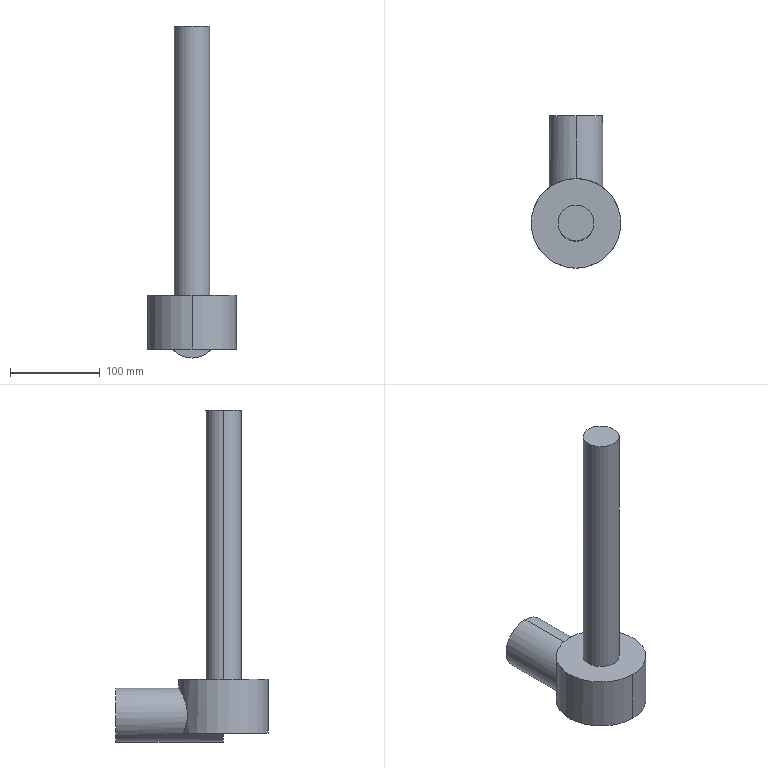Part | SolidWorks | 1 solid | 11 faces | box 100 x 170 x 370 mm | volume 1067997 mm3 | cylinder 6 | plane 5 | commonest cylinder face diameters 40 x2 60 x2 100 x2
STEP:
#1=CARTESIAN_POINT('',(20.,0.,340.));
#2=VERTEX_POINT('',#1);
#3=CARTESIAN_POINT('',(-20.,0.,340.));
#4=VERTEX_POINT('',#3);
#5=CARTESIAN_POINT('',(0.,0.,340.));
#6=DIRECTION('',(0.,0.,1.));
#7=DIRECTION('',(1.,0.,0.));
#8=AXIS2_PLACEMENT_3D('',#5,#6,#7);
#9=CIRCLE('',#8,20.);
#10=EDGE_CURVE('',#2,#4,#9,.T.);
#11=ORIENTED_EDGE('',*,*,#10,.F.);
#12=CARTESIAN_POINT('',(20.,0.,40.));
#13=VERTEX_POINT('',#12);
#14=CARTESIAN_POINT('',(20.,0.,340.));
#15=DIRECTION('',(0.,0.,-1.));
#16=VECTOR('',#15,1000.);
#17=LINE('',#14,#16);
#18=EDGE_CURVE('',#2,#13,#17,.T.);
#19=ORIENTED_EDGE('',*,*,#18,.T.);
#20=CARTESIAN_POINT('',(-20.,0.,40.));
#21=VERTEX_POINT('',#20);
#22=CARTESIAN_POINT('',(0.,0.,40.));
#23=DIRECTION('',(0.,0.,1.));
#24=DIRECTION('',(1.,0.,0.));
#25=AXIS2_PLACEMENT_3D('',#22,#23,#24);
#26=CIRCLE('',#25,20.);
#27=EDGE_CURVE('',#13,#21,#26,.T.);
#28=ORIENTED_EDGE('',*,*,#27,.T.);
#29=CARTESIAN_POINT('',(-20.,0.,340.));
#30=DIRECTION('',(0.,0.,-1.));
#31=VECTOR('',#30,1000.);
#32=LINE('',#29,#31);
#33=EDGE_CURVE('',#4,#21,#32,.T.);
#34=ORIENTED_EDGE('',*,*,#33,.F.);
#35=EDGE_LOOP('',(#11,#19,#28,#34));
#36=FACE_OUTER_BOUND('',#35,.T.);
#37=CARTESIAN_POINT('',(0.,0.,340.));
#38=DIRECTION('',(0.,0.,-1.));
#39=DIRECTION('',(-1.,0.,0.));
#40=AXIS2_PLACEMENT_3D('',#37,#38,#39);
#41=CYLINDRICAL_SURFACE('',#40,20.);
#42=ADVANCED_FACE('',(#36),#41,.T.);
#43=CARTESIAN_POINT('',(0.,50.,30.));
#44=VERTEX_POINT('',#43);
#45=CARTESIAN_POINT('',(22.361,44.721,-20.));
#46=VERTEX_POINT('',#45);
#47=CARTESIAN_POINT('',(0.,50.,30.));
#48=CARTESIAN_POINT('',(1.484,50.,30.));
#49=CARTESIAN_POINT('',(2.949,49.934,29.891));
#50=CARTESIAN_POINT('',(5.122,49.742,29.569));
#51=CARTESIAN_POINT('',(5.841,49.663,29.435));
#52=CARTESIAN_POINT('',(7.272,49.474,29.114));
#53=CARTESIAN_POINT('',(7.986,49.363,28.927));
#54=CARTESIAN_POINT('',(10.089,48.992,28.291));
#55=CARTESIAN_POINT('',(11.436,48.693,27.772));
#56=CARTESIAN_POINT('',(13.383,48.18,26.859));
#57=CARTESIAN_POINT('',(14.019,47.999,26.533));
#58=CARTESIAN_POINT('',(15.267,47.617,25.835));
#59=CARTESIAN_POINT('',(15.881,47.415,25.462));
#60=CARTESIAN_POINT('',(17.667,46.792,24.288));
#61=CARTESIAN_POINT('',(18.784,46.351,23.433));
#62=CARTESIAN_POINT('',(20.886,45.443,21.581));
#63=CARTESIAN_POINT('',(21.869,44.975,20.585));
#64=CARTESIAN_POINT('',(23.705,44.036,18.441));
#65=CARTESIAN_POINT('',(24.54,43.573,17.314));
#66=CARTESIAN_POINT('',(26.045,42.69,14.953));
#67=CARTESIAN_POINT('',(26.718,42.269,13.718));
#68=CARTESIAN_POINT('',(27.602,41.692,11.775));
#69=CARTESIAN_POINT('',(27.876,41.509,11.112));
#70=CARTESIAN_POINT('',(28.38,41.166,9.752));
#71=CARTESIAN_POINT('',(28.607,41.008,9.063));
#72=CARTESIAN_POINT('',(29.213,40.581,6.977));
#73=CARTESIAN_POINT('',(29.518,40.358,5.555));
#74=CARTESIAN_POINT('',(29.819,40.135,3.371));
#75=CARTESIAN_POINT('',(29.894,40.08,2.632));
#76=CARTESIAN_POINT('',(29.987,40.01,1.146));
#77=CARTESIAN_POINT('',(30.006,39.995,0.4062));
#78=CARTESIAN_POINT('',(29.982,40.014,-1.804));
#79=CARTESIAN_POINT('',(29.858,40.107,-3.265));
#80=CARTESIAN_POINT('',(29.512,40.362,-5.44));
#81=CARTESIAN_POINT('',(29.369,40.466,-6.164));
#82=CARTESIAN_POINT('',(29.032,40.708,-7.594));
#83=CARTESIAN_POINT('',(28.839,40.846,-8.295));
#84=CARTESIAN_POINT('',(28.19,41.299,-10.365));
#85=CARTESIAN_POINT('',(27.663,41.657,-11.696));
#86=CARTESIAN_POINT('',(26.735,42.254,-13.629));
#87=CARTESIAN_POINT('',(26.402,42.463,-14.263));
#88=CARTESIAN_POINT('',(25.698,42.893,-15.496));
#89=CARTESIAN_POINT('',(25.326,43.114,-16.096));
#90=CARTESIAN_POINT('',(24.154,43.788,-17.848));
#91=CARTESIAN_POINT('',(23.297,44.253,-18.953));
#92=CARTESIAN_POINT('',(22.361,44.721,-20.));
#93=B_SPLINE_CURVE_WITH_KNOTS('',3,(#47,#48,#49,#50,#51,#52,#53,#54,#55,#56,#57,#58,#59,#60,#61,#62,#63,#64,#65,#66,#67,#68,#69,#70,#71,#72,#73,#74,#75,#76,#77,#78,#79,#80,#81,#82,#83,#84,#85,#86,#87,#88,#89,#90,#91,#92),.UNSPECIFIED.,.F.,.F.,(4,2,2,2,2,2,2,2,2,2,2,2,2,2,2,2,2,2,2,2,2,2,4),(0.09625,0.1006,0.1028,0.105,0.1094,0.1116,0.1138,0.1182,0.1226,0.127,0.1314,0.1336,0.1358,0.1402,0.1424,0.1446,0.149,0.1512,0.1534,0.1578,0.16,0.1622,0.1666),.UNSPECIFIED.);
#94=EDGE_CURVE('',#44,#46,#93,.T.);
#95=ORIENTED_EDGE('',*,*,#94,.F.);
#96=CARTESIAN_POINT('',(0.,50.,40.));
#97=VERTEX_POINT('',#96);
#98=CARTESIAN_POINT('',(0.,50.,-20.));
#99=DIRECTION('',(0.,0.,1.));
#100=VECTOR('',#99,1000.);
#101=LINE('',#98,#100);
#102=EDGE_CURVE('',#44,#97,#101,.T.);
#103=ORIENTED_EDGE('',*,*,#102,.T.);
#104=CARTESIAN_POINT('',(0.,-50.,40.));
#105=VERTEX_POINT('',#104);
#106=CARTESIAN_POINT('',(0.,0.,40.));
#107=DIRECTION('',(0.,0.,1.));
#108=DIRECTION('',(0.,-1.,0.));
#109=AXIS2_PLACEMENT_3D('',#106,#107,#108);
#110=CIRCLE('',#109,50.);
#111=EDGE_CURVE('',#105,#97,#110,.T.);
#112=ORIENTED_EDGE('',*,*,#111,.F.);
#113=CARTESIAN_POINT('',(0.,-50.,-20.));
#114=VERTEX_POINT('',#113);
#115=CARTESIAN_POINT('',(0.,-50.,-20.));
#116=DIRECTION('',(0.,0.,1.));
#117=VECTOR('',#116,1000.);
#118=LINE('',#115,#117);
#119=EDGE_CURVE('',#114,#105,#118,.T.);
#120=ORIENTED_EDGE('',*,*,#119,.F.);
#121=CARTESIAN_POINT('',(0.,0.,-20.));
#122=DIRECTION('',(0.,0.,1.));
#123=DIRECTION('',(0.,-1.,0.));
#124=AXIS2_PLACEMENT_3D('',#121,#122,#123);
#125=CIRCLE('',#124,50.);
#126=EDGE_CURVE('',#114,#46,#125,.T.);
#127=ORIENTED_EDGE('',*,*,#126,.T.);
#128=EDGE_LOOP('',(#95,#103,#112,#120,#127));
#129=FACE_OUTER_BOUND('',#128,.T.);
#130=CARTESIAN_POINT('',(0.,0.,-20.));
#131=DIRECTION('',(0.,0.,1.));
#132=DIRECTION('',(0.,-1.,0.));
#133=AXIS2_PLACEMENT_3D('',#130,#131,#132);
#134=CYLINDRICAL_SURFACE('',#133,50.);
#135=ADVANCED_FACE('',(#129),#134,.T.);
#136=CARTESIAN_POINT('',(0.,120.,30.));
#137=VERTEX_POINT('',#136);
#138=CARTESIAN_POINT('',(0.,120.,-30.));
#139=VERTEX_POINT('',#138);
#140=CARTESIAN_POINT('',(0.,120.,0.));
#141=DIRECTION('',(0.,1.,0.));
#142=DIRECTION('',(0.,0.,1.));
#143=AXIS2_PLACEMENT_3D('',#140,#141,#142);
#144=CIRCLE('',#143,30.);
#145=EDGE_CURVE('',#137,#139,#144,.T.);
#146=ORIENTED_EDGE('',*,*,#145,.F.);
#147=CARTESIAN_POINT('',(0.,120.,30.));
#148=DIRECTION('',(0.,-1.,0.));
#149=VECTOR('',#148,1000.);
#150=LINE('',#147,#149);
#151=EDGE_CURVE('',#137,#44,#150,.T.);
#152=ORIENTED_EDGE('',*,*,#151,.T.);
#153=ORIENTED_EDGE('',*,*,#94,.T.);
#154=CARTESIAN_POINT('',(22.361,0.,-20.));
#155=VERTEX_POINT('',#154);
#156=CARTESIAN_POINT('',(22.361,120.,-20.));
#157=DIRECTION('',(0.,1.,0.));
#158=VECTOR('',#157,1000.);
#159=LINE('',#156,#158);
#160=EDGE_CURVE('',#155,#46,#159,.T.);
#161=ORIENTED_EDGE('',*,*,#160,.F.);
#162=CARTESIAN_POINT('',(0.,0.,-30.));
#163=VERTEX_POINT('',#162);
#164=CARTESIAN_POINT('',(0.,0.,0.));
#165=DIRECTION('',(0.,1.,0.));
#166=DIRECTION('',(0.,0.,1.));
#167=AXIS2_PLACEMENT_3D('',#164,#165,#166);
#168=CIRCLE('',#167,30.);
#169=EDGE_CURVE('',#155,#163,#168,.T.);
#170=ORIENTED_EDGE('',*,*,#169,.T.);
#171=CARTESIAN_POINT('',(0.,120.,-30.));
#172=DIRECTION('',(0.,-1.,0.));
#173=VECTOR('',#172,1000.);
#174=LINE('',#171,#173);
#175=EDGE_CURVE('',#139,#163,#174,.T.);
#176=ORIENTED_EDGE('',*,*,#175,.F.);
#177=EDGE_LOOP('',(#146,#152,#153,#161,#170,#176));
#178=FACE_OUTER_BOUND('',#177,.T.);
#179=CARTESIAN_POINT('',(0.,120.,0.));
#180=DIRECTION('',(0.,-1.,0.));
#181=DIRECTION('',(0.,0.,-1.));
#182=AXIS2_PLACEMENT_3D('',#179,#180,#181);
#183=CYLINDRICAL_SURFACE('',#182,30.);
#184=ADVANCED_FACE('',(#178),#183,.T.);
#185=ORIENTED_EDGE('',*,*,#151,.F.);
#186=CARTESIAN_POINT('',(0.,120.,0.));
#187=DIRECTION('',(0.,1.,0.));
#188=DIRECTION('',(0.,0.,1.));
#189=AXIS2_PLACEMENT_3D('',#186,#187,#188);
#190=CIRCLE('',#189,30.);
#191=EDGE_CURVE('',#139,#137,#190,.T.);
#192=ORIENTED_EDGE('',*,*,#191,.F.);
#193=ORIENTED_EDGE('',*,*,#175,.T.);
#194=CARTESIAN_POINT('',(-22.361,0.,-20.));
#195=VERTEX_POINT('',#194);
#196=CARTESIAN_POINT('',(0.,0.,0.));
#197=DIRECTION('',(0.,1.,0.));
#198=DIRECTION('',(0.,0.,1.));
#199=AXIS2_PLACEMENT_3D('',#196,#197,#198);
#200=CIRCLE('',#199,30.);
#201=EDGE_CURVE('',#163,#195,#200,.T.);
#202=ORIENTED_EDGE('',*,*,#201,.T.);
#203=CARTESIAN_POINT('',(-22.361,44.721,-20.));
#204=VERTEX_POINT('',#203);
#205=CARTESIAN_POINT('',(-22.361,120.,-20.));
#206=DIRECTION('',(0.,-1.,0.));
#207=VECTOR('',#206,1000.);
#208=LINE('',#205,#207);
#209=EDGE_CURVE('',#204,#195,#208,.T.);
#210=ORIENTED_EDGE('',*,*,#209,.F.);
#211=CARTESIAN_POINT('',(-22.361,44.721,-20.));
#212=CARTESIAN_POINT('',(-22.828,44.488,-19.478));
#213=CARTESIAN_POINT('',(-23.277,44.254,-18.938));
#214=CARTESIAN_POINT('',(-24.143,43.788,-17.822));
#215=CARTESIAN_POINT('',(-24.555,43.558,-17.25));
#216=CARTESIAN_POINT('',(-25.726,42.884,-15.497));
#217=CARTESIAN_POINT('',(-26.422,42.455,-14.279));
#218=CARTESIAN_POINT('',(-27.646,41.668,-11.733));
#219=CARTESIAN_POINT('',(-28.175,41.309,-10.406));
#220=CARTESIAN_POINT('',(-28.832,40.851,-8.321));
#221=CARTESIAN_POINT('',(-29.026,40.713,-7.616));
#222=CARTESIAN_POINT('',(-29.362,40.471,-6.197));
#223=CARTESIAN_POINT('',(-29.504,40.367,-5.481));
#224=CARTESIAN_POINT('',(-29.736,40.197,-4.038));
#225=CARTESIAN_POINT('',(-29.826,40.13,-3.31));
#226=CARTESIAN_POINT('',(-29.953,40.036,-1.841));
#227=CARTESIAN_POINT('',(-29.989,40.008,-1.098));
#228=CARTESIAN_POINT('',(-30.015,39.988,1.139));
#229=CARTESIAN_POINT('',(-29.922,40.059,2.61));
#230=CARTESIAN_POINT('',(-29.625,40.279,4.786));
#231=CARTESIAN_POINT('',(-29.499,40.371,5.507));
#232=CARTESIAN_POINT('',(-29.196,40.591,6.939));
#233=CARTESIAN_POINT('',(-29.017,40.72,7.653));
#234=CARTESIAN_POINT('',(-28.407,41.149,9.755));
#235=CARTESIAN_POINT('',(-27.907,41.494,11.102));
#236=CARTESIAN_POINT('',(-27.023,42.07,13.05));
#237=CARTESIAN_POINT('',(-26.705,42.273,13.687));
#238=CARTESIAN_POINT('',(-26.026,42.694,14.938));
#239=CARTESIAN_POINT('',(-25.663,42.914,15.553));
#240=CARTESIAN_POINT('',(-24.522,43.583,17.34));
#241=CARTESIAN_POINT('',(-23.686,44.046,18.465));
#242=CARTESIAN_POINT('',(-22.32,44.744,20.057));
#243=CARTESIAN_POINT('',(-21.846,44.978,20.573));
#244=CARTESIAN_POINT('',(-20.86,45.444,21.572));
#245=CARTESIAN_POINT('',(-20.346,45.677,22.058));
#246=CARTESIAN_POINT('',(-18.752,46.365,23.46));
#247=CARTESIAN_POINT('',(-17.633,46.804,24.312));
#248=CARTESIAN_POINT('',(-15.277,47.625,25.858));
#249=CARTESIAN_POINT('',(-14.04,48.007,26.551));
#250=CARTESIAN_POINT('',(-12.089,48.521,27.466));
#251=CARTESIAN_POINT('',(-11.421,48.683,27.75));
#252=CARTESIAN_POINT('',(-10.058,48.983,28.273));
#253=CARTESIAN_POINT('',(-9.37,49.119,28.508));
#254=CARTESIAN_POINT('',(-7.284,49.487,29.139));
#255=CARTESIAN_POINT('',(-5.866,49.676,29.457));
#256=CARTESIAN_POINT('',(-3.697,49.868,29.78));
#257=CARTESIAN_POINT('',(-2.967,49.917,29.862));
#258=CARTESIAN_POINT('',(-1.492,49.983,29.972));
#259=CARTESIAN_POINT('',(-0.7434,50.,30.));
#260=CARTESIAN_POINT('',(0.,50.,30.));
#261=B_SPLINE_CURVE_WITH_KNOTS('',3,(#211,#212,#213,#214,#215,#216,#217,#218,#219,#220,#221,#222,#223,#224,#225,#226,#227,#228,#229,#230,#231,#232,#233,#234,#235,#236,#237,#238,#239,#240,#241,#242,#243,#244,#245,#246,#247,#248,#249,#250,#251,#252,#253,#254,#255,#256,#257,#258,#259,#260),.UNSPECIFIED.,.F.,.F.,(4,2,2,2,2,2,2,2,2,2,2,2,2,2,2,2,2,2,2,2,2,2,2,2,4),(0.02576,0.02796,0.03017,0.03457,0.03898,0.04118,0.04338,0.04558,0.04779,0.05219,0.0544,0.0566,0.061,0.06321,0.06541,0.06981,0.07202,0.07422,0.07863,0.08303,0.08523,0.08744,0.09184,0.09404,0.09625),.UNSPECIFIED.);
#262=EDGE_CURVE('',#204,#44,#261,.T.);
#263=ORIENTED_EDGE('',*,*,#262,.T.);
#264=EDGE_LOOP('',(#185,#192,#193,#202,#210,#263));
#265=FACE_OUTER_BOUND('',#264,.T.);
#266=CARTESIAN_POINT('',(0.,120.,0.));
#267=DIRECTION('',(0.,-1.,0.));
#268=DIRECTION('',(0.,0.,-1.));
#269=AXIS2_PLACEMENT_3D('',#266,#267,#268);
#270=CYLINDRICAL_SURFACE('',#269,30.);
#271=ADVANCED_FACE('',(#265),#270,.T.);
#272=CARTESIAN_POINT('',(0.,0.,-20.));
#273=DIRECTION('',(1.,0.,0.));
#274=VECTOR('',#273,1000.);
#275=LINE('',#272,#274);
#276=EDGE_CURVE('',#195,#155,#275,.T.);
#277=ORIENTED_EDGE('',*,*,#276,.F.);
#278=ORIENTED_EDGE('',*,*,#201,.F.);
#279=ORIENTED_EDGE('',*,*,#169,.F.);
#280=EDGE_LOOP('',(#277,#278,#279));
#281=FACE_OUTER_BOUND('',#280,.T.);
#282=CARTESIAN_POINT('',(0.,0.,0.));
#283=DIRECTION('',(0.,1.,0.));
#284=DIRECTION('',(0.,0.,1.));
#285=AXIS2_PLACEMENT_3D('',#282,#283,#284);
#286=PLANE('',#285);
#287=ADVANCED_FACE('',(#281),#286,.F.);
#288=ORIENTED_EDGE('',*,*,#191,.T.);
#289=ORIENTED_EDGE('',*,*,#145,.T.);
#290=EDGE_LOOP('',(#288,#289));
#291=FACE_OUTER_BOUND('',#290,.T.);
#292=CARTESIAN_POINT('',(0.,120.,0.));
#293=DIRECTION('',(0.,1.,0.));
#294=DIRECTION('',(0.,0.,1.));
#295=AXIS2_PLACEMENT_3D('',#292,#293,#294);
#296=PLANE('',#295);
#297=ADVANCED_FACE('',(#291),#296,.T.);
#298=ORIENTED_EDGE('',*,*,#102,.F.);
#299=ORIENTED_EDGE('',*,*,#262,.F.);
#300=CARTESIAN_POINT('',(0.,0.,-20.));
#301=DIRECTION('',(0.,0.,1.));
#302=DIRECTION('',(0.,-1.,0.));
#303=AXIS2_PLACEMENT_3D('',#300,#301,#302);
#304=CIRCLE('',#303,50.);
#305=EDGE_CURVE('',#204,#114,#304,.T.);
#306=ORIENTED_EDGE('',*,*,#305,.T.);
#307=ORIENTED_EDGE('',*,*,#119,.T.);
#308=CARTESIAN_POINT('',(0.,0.,40.));
#309=DIRECTION('',(0.,0.,1.));
#310=DIRECTION('',(0.,-1.,0.));
#311=AXIS2_PLACEMENT_3D('',#308,#309,#310);
#312=CIRCLE('',#311,50.);
#313=EDGE_CURVE('',#97,#105,#312,.T.);
#314=ORIENTED_EDGE('',*,*,#313,.F.);
#315=EDGE_LOOP('',(#298,#299,#306,#307,#314));
#316=FACE_OUTER_BOUND('',#315,.T.);
#317=CARTESIAN_POINT('',(0.,0.,-20.));
#318=DIRECTION('',(0.,0.,1.));
#319=DIRECTION('',(0.,-1.,0.));
#320=AXIS2_PLACEMENT_3D('',#317,#318,#319);
#321=CYLINDRICAL_SURFACE('',#320,50.);
#322=ADVANCED_FACE('',(#316),#321,.T.);
#323=ORIENTED_EDGE('',*,*,#305,.F.);
#324=ORIENTED_EDGE('',*,*,#209,.T.);
#325=ORIENTED_EDGE('',*,*,#276,.T.);
#326=ORIENTED_EDGE('',*,*,#160,.T.);
#327=ORIENTED_EDGE('',*,*,#126,.F.);
#328=EDGE_LOOP('',(#323,#324,#325,#326,#327));
#329=FACE_OUTER_BOUND('',#328,.T.);
#330=CARTESIAN_POINT('',(0.,0.,-20.));
#331=DIRECTION('',(0.,0.,1.));
#332=DIRECTION('',(0.,-1.,0.));
#333=AXIS2_PLACEMENT_3D('',#330,#331,#332);
#334=PLANE('',#333);
#335=ADVANCED_FACE('',(#329),#334,.F.);
#336=CARTESIAN_POINT('',(0.,0.,40.));
#337=DIRECTION('',(0.,0.,1.));
#338=DIRECTION('',(1.,0.,0.));
#339=AXIS2_PLACEMENT_3D('',#336,#337,#338);
#340=CIRCLE('',#339,20.);
#341=EDGE_CURVE('',#21,#13,#340,.T.);
#342=ORIENTED_EDGE('',*,*,#341,.F.);
#343=ORIENTED_EDGE('',*,*,#27,.F.);
#344=EDGE_LOOP('',(#342,#343));
#345=FACE_BOUND('',#344,.T.);
#346=ORIENTED_EDGE('',*,*,#111,.T.);
#347=ORIENTED_EDGE('',*,*,#313,.T.);
#348=EDGE_LOOP('',(#346,#347));
#349=FACE_OUTER_BOUND('',#348,.T.);
#350=CARTESIAN_POINT('',(0.,0.,40.));
#351=DIRECTION('',(0.,0.,1.));
#352=DIRECTION('',(0.,-1.,0.));
#353=AXIS2_PLACEMENT_3D('',#350,#351,#352);
#354=PLANE('',#353);
#355=ADVANCED_FACE('',(#345,#349),#354,.T.);
#356=ORIENTED_EDGE('',*,*,#18,.F.);
#357=CARTESIAN_POINT('',(0.,0.,340.));
#358=DIRECTION('',(0.,0.,1.));
#359=DIRECTION('',(1.,0.,0.));
#360=AXIS2_PLACEMENT_3D('',#357,#358,#359);
#361=CIRCLE('',#360,20.);
#362=EDGE_CURVE('',#4,#2,#361,.T.);
#363=ORIENTED_EDGE('',*,*,#362,.F.);
#364=ORIENTED_EDGE('',*,*,#33,.T.);
#365=ORIENTED_EDGE('',*,*,#341,.T.);
#366=EDGE_LOOP('',(#356,#363,#364,#365));
#367=FACE_OUTER_BOUND('',#366,.T.);
#368=CARTESIAN_POINT('',(0.,0.,340.));
#369=DIRECTION('',(0.,0.,-1.));
#370=DIRECTION('',(-1.,0.,0.));
#371=AXIS2_PLACEMENT_3D('',#368,#369,#370);
#372=CYLINDRICAL_SURFACE('',#371,20.);
#373=ADVANCED_FACE('',(#367),#372,.T.);
#374=ORIENTED_EDGE('',*,*,#362,.T.);
#375=ORIENTED_EDGE('',*,*,#10,.T.);
#376=EDGE_LOOP('',(#374,#375));
#377=FACE_OUTER_BOUND('',#376,.T.);
#378=CARTESIAN_POINT('',(0.,0.,340.));
#379=DIRECTION('',(0.,0.,1.));
#380=DIRECTION('',(1.,0.,0.));
#381=AXIS2_PLACEMENT_3D('',#378,#379,#380);
#382=PLANE('',#381);
#383=ADVANCED_FACE('',(#377),#382,.T.);
#384=CLOSED_SHELL('',(#42,#135,#184,#271,#287,#297,#322,#335,#355,#373,#383));
#385=MANIFOLD_SOLID_BREP('',#384);
#386=CARTESIAN_POINT('',(0.,0.,0.));
#387=DIRECTION('',(0.,0.,1.));
#388=DIRECTION('',(1.,0.,0.));
#389=AXIS2_PLACEMENT_3D('',#386,#387,#388);
#390=(LENGTH_UNIT()NAMED_UNIT(*)SI_UNIT(.MILLI.,.METRE.));
#391=UNCERTAINTY_MEASURE_WITH_UNIT(LENGTH_MEASURE(0.00001),#390,'','');
#392=(NAMED_UNIT(*)PLANE_ANGLE_UNIT()SI_UNIT($,.RADIAN.));
#393=(NAMED_UNIT(*)SI_UNIT($,.STERADIAN.)SOLID_ANGLE_UNIT());
#394=(GEOMETRIC_REPRESENTATION_CONTEXT(3)GLOBAL_UNCERTAINTY_ASSIGNED_CONTEXT((#391))GLOBAL_UNIT_ASSIGNED_CONTEXT((#390,#392,#393))REPRESENTATION_CONTEXT('',''));
#395=ADVANCED_BREP_SHAPE_REPRESENTATION('',(#385,#389),#394);